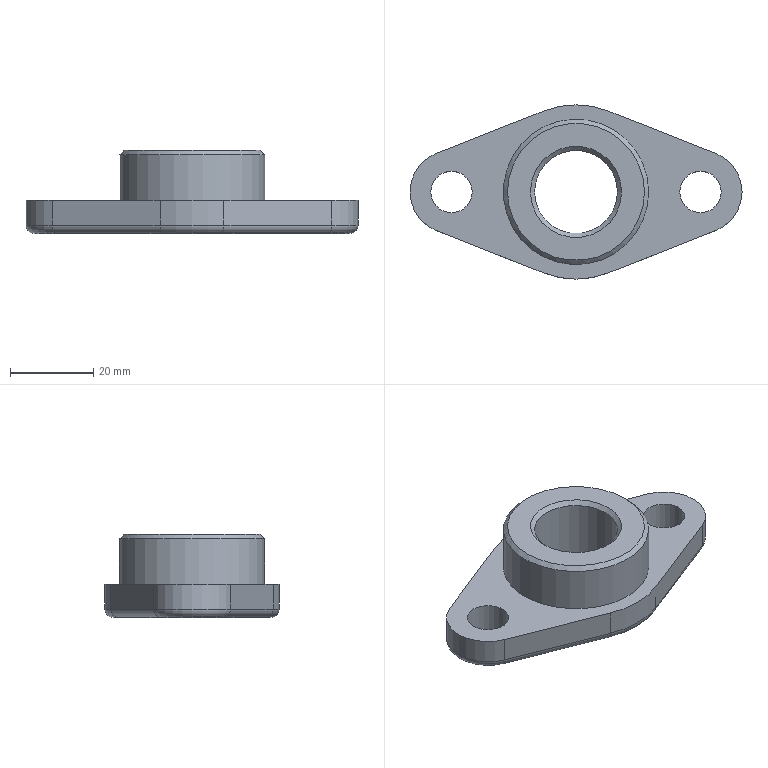Part | NX | features DATUM_CSYS 3, EXTRUDE 2, SKETCH 2, BLEND 1, CHAMFER 1, REPLACE_FACE 1 | 1 solid | 28 faces | box 80 x 42 x 20 mm | volume 22097 mm3 | cylinder 12 | plane 7 | cone 5 | torus 4 | commonest cylinder face diameters 4 x4 20 x3 10 x2 42 x2 35 x1
STEP:
#1=CARTESIAN_POINT('',(32.933,7.443,0.));
#2=VERTEX_POINT('',#1);
#3=CARTESIAN_POINT('',(32.933,-7.443,0.));
#4=VERTEX_POINT('',#3);
#5=CARTESIAN_POINT('',(30.,0.,0.));
#6=DIRECTION('',(0.,0.,1.));
#7=DIRECTION('',(1.,0.,0.));
#8=AXIS2_PLACEMENT_3D('',#5,#6,#7);
#9=CIRCLE('',#8,8.);
#10=EDGE_CURVE('',#2,#4,#9,.F.);
#11=ORIENTED_EDGE('',*,*,#10,.T.);
#12=CARTESIAN_POINT('',(6.967,-17.677,0.));
#13=VERTEX_POINT('',#12);
#14=CARTESIAN_POINT('',(-19.,-27.911,0.));
#15=DIRECTION('',(0.9304,0.3667,0.));
#16=VECTOR('',#15,1000.);
#17=LINE('',#14,#16);
#18=EDGE_CURVE('',#4,#13,#17,.F.);
#19=ORIENTED_EDGE('',*,*,#18,.T.);
#20=CARTESIAN_POINT('',(-6.967,-17.677,0.));
#21=VERTEX_POINT('',#20);
#22=CARTESIAN_POINT('',(0.,0.,0.));
#23=DIRECTION('',(0.,0.,1.));
#24=DIRECTION('',(1.,0.,0.));
#25=AXIS2_PLACEMENT_3D('',#22,#23,#24);
#26=CIRCLE('',#25,19.);
#27=EDGE_CURVE('',#13,#21,#26,.F.);
#28=ORIENTED_EDGE('',*,*,#27,.T.);
#29=CARTESIAN_POINT('',(-32.933,-7.443,0.));
#30=VERTEX_POINT('',#29);
#31=CARTESIAN_POINT('',(-32.933,-7.443,0.));
#32=DIRECTION('',(0.9304,-0.3667,0.));
#33=VECTOR('',#32,1000.);
#34=LINE('',#31,#33);
#35=EDGE_CURVE('',#21,#30,#34,.F.);
#36=ORIENTED_EDGE('',*,*,#35,.T.);
#37=CARTESIAN_POINT('',(-32.933,7.443,0.));
#38=VERTEX_POINT('',#37);
#39=CARTESIAN_POINT('',(-30.,0.,0.));
#40=DIRECTION('',(0.,0.,1.));
#41=DIRECTION('',(1.,0.,0.));
#42=AXIS2_PLACEMENT_3D('',#39,#40,#41);
#43=CIRCLE('',#42,8.);
#44=EDGE_CURVE('',#30,#38,#43,.F.);
#45=ORIENTED_EDGE('',*,*,#44,.T.);
#46=CARTESIAN_POINT('',(-6.967,17.677,0.));
#47=VERTEX_POINT('',#46);
#48=CARTESIAN_POINT('',(-32.933,7.443,0.));
#49=DIRECTION('',(-0.9304,-0.3667,0.));
#50=VECTOR('',#49,1000.);
#51=LINE('',#48,#50);
#52=EDGE_CURVE('',#38,#47,#51,.F.);
#53=ORIENTED_EDGE('',*,*,#52,.T.);
#54=CARTESIAN_POINT('',(6.967,17.677,0.));
#55=VERTEX_POINT('',#54);
#56=CARTESIAN_POINT('',(0.,0.,0.));
#57=DIRECTION('',(0.,0.,1.));
#58=DIRECTION('',(1.,0.,0.));
#59=AXIS2_PLACEMENT_3D('',#56,#57,#58);
#60=CIRCLE('',#59,19.);
#61=EDGE_CURVE('',#47,#55,#60,.F.);
#62=ORIENTED_EDGE('',*,*,#61,.T.);
#63=CARTESIAN_POINT('',(-19.,27.911,0.));
#64=DIRECTION('',(-0.9304,0.3667,0.));
#65=VECTOR('',#64,1000.);
#66=LINE('',#63,#65);
#67=EDGE_CURVE('',#55,#2,#66,.F.);
#68=ORIENTED_EDGE('',*,*,#67,.T.);
#69=EDGE_LOOP('',(#11,#19,#28,#36,#45,#53,#62,#68));
#70=FACE_BOUND('',#69,.T.);
#71=CARTESIAN_POINT('',(11.,0.,0.));
#72=VERTEX_POINT('',#71);
#73=CARTESIAN_POINT('',(0.,0.,0.));
#74=DIRECTION('',(0.,0.,1.));
#75=DIRECTION('',(1.,0.,0.));
#76=AXIS2_PLACEMENT_3D('',#73,#74,#75);
#77=CIRCLE('',#76,11.);
#78=EDGE_CURVE('',#72,#72,#77,.T.);
#79=ORIENTED_EDGE('',*,*,#78,.T.);
#80=EDGE_LOOP('',(#79));
#81=FACE_BOUND('',#80,.T.);
#82=CARTESIAN_POINT('',(36.,0.,0.));
#83=VERTEX_POINT('',#82);
#84=CARTESIAN_POINT('',(30.,0.,0.));
#85=DIRECTION('',(0.,0.,1.));
#86=DIRECTION('',(1.,0.,0.));
#87=AXIS2_PLACEMENT_3D('',#84,#85,#86);
#88=CIRCLE('',#87,6.);
#89=EDGE_CURVE('',#83,#83,#88,.T.);
#90=ORIENTED_EDGE('',*,*,#89,.T.);
#91=EDGE_LOOP('',(#90));
#92=FACE_BOUND('',#91,.T.);
#93=CARTESIAN_POINT('',(-24.,0.,0.));
#94=VERTEX_POINT('',#93);
#95=CARTESIAN_POINT('',(-30.,0.,0.));
#96=DIRECTION('',(0.,0.,1.));
#97=DIRECTION('',(1.,0.,0.));
#98=AXIS2_PLACEMENT_3D('',#95,#96,#97);
#99=CIRCLE('',#98,6.);
#100=EDGE_CURVE('',#94,#94,#99,.T.);
#101=ORIENTED_EDGE('',*,*,#100,.T.);
#102=EDGE_LOOP('',(#101));
#103=FACE_BOUND('',#102,.T.);
#104=CARTESIAN_POINT('',(-30.,0.,0.));
#105=DIRECTION('',(0.,0.,1.));
#106=DIRECTION('',(1.,0.,0.));
#107=AXIS2_PLACEMENT_3D('',#104,#105,#106);
#108=PLANE('',#107);
#109=ADVANCED_FACE('',(#70,#81,#92,#103),#108,.F.);
#110=CARTESIAN_POINT('',(-33.667,9.304,8.));
#111=VERTEX_POINT('',#110);
#112=CARTESIAN_POINT('',(-33.667,9.304,2.));
#113=VERTEX_POINT('',#112);
#114=CARTESIAN_POINT('',(-33.667,9.304,8.));
#115=DIRECTION('',(0.,0.,-1.));
#116=VECTOR('',#115,1000.);
#117=LINE('',#114,#116);
#118=EDGE_CURVE('',#111,#113,#117,.T.);
#119=ORIENTED_EDGE('',*,*,#118,.T.);
#120=CARTESIAN_POINT('',(-33.667,-9.304,2.));
#121=VERTEX_POINT('',#120);
#122=CARTESIAN_POINT('',(-30.,0.,2.));
#123=DIRECTION('',(0.,0.,1.));
#124=DIRECTION('',(1.,0.,0.));
#125=AXIS2_PLACEMENT_3D('',#122,#123,#124);
#126=CIRCLE('',#125,10.);
#127=EDGE_CURVE('',#113,#121,#126,.T.);
#128=ORIENTED_EDGE('',*,*,#127,.T.);
#129=CARTESIAN_POINT('',(-33.667,-9.304,8.));
#130=VERTEX_POINT('',#129);
#131=CARTESIAN_POINT('',(-33.667,-9.304,8.));
#132=DIRECTION('',(0.,0.,-1.));
#133=VECTOR('',#132,1000.);
#134=LINE('',#131,#133);
#135=EDGE_CURVE('',#130,#121,#134,.T.);
#136=ORIENTED_EDGE('',*,*,#135,.F.);
#137=CARTESIAN_POINT('',(-30.,0.,8.));
#138=DIRECTION('',(0.,0.,1.));
#139=DIRECTION('',(1.,0.,0.));
#140=AXIS2_PLACEMENT_3D('',#137,#138,#139);
#141=CIRCLE('',#140,10.);
#142=EDGE_CURVE('',#111,#130,#141,.T.);
#143=ORIENTED_EDGE('',*,*,#142,.F.);
#144=EDGE_LOOP('',(#119,#128,#136,#143));
#145=FACE_BOUND('',#144,.T.);
#146=CARTESIAN_POINT('',(-30.,0.,8.));
#147=DIRECTION('',(0.,0.,-1.));
#148=DIRECTION('',(-1.,0.,0.));
#149=AXIS2_PLACEMENT_3D('',#146,#147,#148);
#150=CYLINDRICAL_SURFACE('',#149,10.);
#151=ADVANCED_FACE('',(#145),#150,.T.);
#152=ORIENTED_EDGE('',*,*,#135,.T.);
#153=CARTESIAN_POINT('',(-7.7,-19.537,2.));
#154=VERTEX_POINT('',#153);
#155=CARTESIAN_POINT('',(-33.667,-9.304,2.));
#156=DIRECTION('',(0.9304,-0.3667,0.));
#157=VECTOR('',#156,1000.);
#158=LINE('',#155,#157);
#159=EDGE_CURVE('',#121,#154,#158,.T.);
#160=ORIENTED_EDGE('',*,*,#159,.T.);
#161=CARTESIAN_POINT('',(-7.7,-19.537,8.));
#162=VERTEX_POINT('',#161);
#163=CARTESIAN_POINT('',(-7.7,-19.537,8.));
#164=DIRECTION('',(0.,0.,-1.));
#165=VECTOR('',#164,1000.);
#166=LINE('',#163,#165);
#167=EDGE_CURVE('',#162,#154,#166,.T.);
#168=ORIENTED_EDGE('',*,*,#167,.F.);
#169=CARTESIAN_POINT('',(-33.667,-9.304,8.));
#170=DIRECTION('',(0.9304,-0.3667,0.));
#171=VECTOR('',#170,1000.);
#172=LINE('',#169,#171);
#173=EDGE_CURVE('',#130,#162,#172,.T.);
#174=ORIENTED_EDGE('',*,*,#173,.F.);
#175=EDGE_LOOP('',(#152,#160,#168,#174));
#176=FACE_BOUND('',#175,.T.);
#177=CARTESIAN_POINT('',(-33.667,-9.304,8.));
#178=DIRECTION('',(0.3667,0.9304,0.));
#179=DIRECTION('',(-0.9304,0.3667,0.));
#180=AXIS2_PLACEMENT_3D('',#177,#178,#179);
#181=PLANE('',#180);
#182=ADVANCED_FACE('',(#176),#181,.F.);
#183=ORIENTED_EDGE('',*,*,#167,.T.);
#184=CARTESIAN_POINT('',(7.7,-19.537,2.));
#185=VERTEX_POINT('',#184);
#186=CARTESIAN_POINT('',(0.,0.,2.));
#187=DIRECTION('',(0.,0.,1.));
#188=DIRECTION('',(1.,0.,0.));
#189=AXIS2_PLACEMENT_3D('',#186,#187,#188);
#190=CIRCLE('',#189,21.);
#191=EDGE_CURVE('',#154,#185,#190,.T.);
#192=ORIENTED_EDGE('',*,*,#191,.T.);
#193=CARTESIAN_POINT('',(7.7,-19.537,8.));
#194=VERTEX_POINT('',#193);
#195=CARTESIAN_POINT('',(7.7,-19.537,8.));
#196=DIRECTION('',(0.,0.,-1.));
#197=VECTOR('',#196,1000.);
#198=LINE('',#195,#197);
#199=EDGE_CURVE('',#194,#185,#198,.T.);
#200=ORIENTED_EDGE('',*,*,#199,.F.);
#201=CARTESIAN_POINT('',(0.,0.,8.));
#202=DIRECTION('',(0.,0.,1.));
#203=DIRECTION('',(1.,0.,0.));
#204=AXIS2_PLACEMENT_3D('',#201,#202,#203);
#205=CIRCLE('',#204,21.);
#206=EDGE_CURVE('',#162,#194,#205,.T.);
#207=ORIENTED_EDGE('',*,*,#206,.F.);
#208=EDGE_LOOP('',(#183,#192,#200,#207));
#209=FACE_BOUND('',#208,.T.);
#210=CARTESIAN_POINT('',(0.,0.,8.));
#211=DIRECTION('',(0.,0.,-1.));
#212=DIRECTION('',(-1.,0.,0.));
#213=AXIS2_PLACEMENT_3D('',#210,#211,#212);
#214=CYLINDRICAL_SURFACE('',#213,21.);
#215=ADVANCED_FACE('',(#209),#214,.T.);
#216=ORIENTED_EDGE('',*,*,#199,.T.);
#217=CARTESIAN_POINT('',(33.667,-9.304,2.));
#218=VERTEX_POINT('',#217);
#219=CARTESIAN_POINT('',(7.7,-19.537,2.));
#220=DIRECTION('',(0.9304,0.3667,0.));
#221=VECTOR('',#220,1000.);
#222=LINE('',#219,#221);
#223=EDGE_CURVE('',#185,#218,#222,.T.);
#224=ORIENTED_EDGE('',*,*,#223,.T.);
#225=CARTESIAN_POINT('',(33.667,-9.304,8.));
#226=VERTEX_POINT('',#225);
#227=CARTESIAN_POINT('',(33.667,-9.304,8.));
#228=DIRECTION('',(0.,0.,-1.));
#229=VECTOR('',#228,1000.);
#230=LINE('',#227,#229);
#231=EDGE_CURVE('',#226,#218,#230,.T.);
#232=ORIENTED_EDGE('',*,*,#231,.F.);
#233=CARTESIAN_POINT('',(7.7,-19.537,8.));
#234=DIRECTION('',(0.9304,0.3667,0.));
#235=VECTOR('',#234,1000.);
#236=LINE('',#233,#235);
#237=EDGE_CURVE('',#194,#226,#236,.T.);
#238=ORIENTED_EDGE('',*,*,#237,.F.);
#239=EDGE_LOOP('',(#216,#224,#232,#238));
#240=FACE_BOUND('',#239,.T.);
#241=CARTESIAN_POINT('',(7.7,-19.537,8.));
#242=DIRECTION('',(-0.3667,0.9304,0.));
#243=DIRECTION('',(-0.9304,-0.3667,0.));
#244=AXIS2_PLACEMENT_3D('',#241,#242,#243);
#245=PLANE('',#244);
#246=ADVANCED_FACE('',(#240),#245,.F.);
#247=ORIENTED_EDGE('',*,*,#231,.T.);
#248=CARTESIAN_POINT('',(33.667,9.304,2.));
#249=VERTEX_POINT('',#248);
#250=CARTESIAN_POINT('',(30.,0.,2.));
#251=DIRECTION('',(0.,0.,1.));
#252=DIRECTION('',(1.,0.,0.));
#253=AXIS2_PLACEMENT_3D('',#250,#251,#252);
#254=CIRCLE('',#253,10.);
#255=EDGE_CURVE('',#218,#249,#254,.T.);
#256=ORIENTED_EDGE('',*,*,#255,.T.);
#257=CARTESIAN_POINT('',(33.667,9.304,8.));
#258=VERTEX_POINT('',#257);
#259=CARTESIAN_POINT('',(33.667,9.304,8.));
#260=DIRECTION('',(0.,0.,-1.));
#261=VECTOR('',#260,1000.);
#262=LINE('',#259,#261);
#263=EDGE_CURVE('',#258,#249,#262,.T.);
#264=ORIENTED_EDGE('',*,*,#263,.F.);
#265=CARTESIAN_POINT('',(30.,0.,8.));
#266=DIRECTION('',(0.,0.,1.));
#267=DIRECTION('',(1.,0.,0.));
#268=AXIS2_PLACEMENT_3D('',#265,#266,#267);
#269=CIRCLE('',#268,10.);
#270=EDGE_CURVE('',#226,#258,#269,.T.);
#271=ORIENTED_EDGE('',*,*,#270,.F.);
#272=EDGE_LOOP('',(#247,#256,#264,#271));
#273=FACE_BOUND('',#272,.T.);
#274=CARTESIAN_POINT('',(30.,0.,8.));
#275=DIRECTION('',(0.,0.,-1.));
#276=DIRECTION('',(-1.,0.,0.));
#277=AXIS2_PLACEMENT_3D('',#274,#275,#276);
#278=CYLINDRICAL_SURFACE('',#277,10.);
#279=ADVANCED_FACE('',(#273),#278,.T.);
#280=ORIENTED_EDGE('',*,*,#263,.T.);
#281=CARTESIAN_POINT('',(7.7,19.537,2.));
#282=VERTEX_POINT('',#281);
#283=CARTESIAN_POINT('',(33.667,9.304,2.));
#284=DIRECTION('',(-0.9304,0.3667,0.));
#285=VECTOR('',#284,1000.);
#286=LINE('',#283,#285);
#287=EDGE_CURVE('',#249,#282,#286,.T.);
#288=ORIENTED_EDGE('',*,*,#287,.T.);
#289=CARTESIAN_POINT('',(7.7,19.537,8.));
#290=VERTEX_POINT('',#289);
#291=CARTESIAN_POINT('',(7.7,19.537,8.));
#292=DIRECTION('',(0.,0.,-1.));
#293=VECTOR('',#292,1000.);
#294=LINE('',#291,#293);
#295=EDGE_CURVE('',#290,#282,#294,.T.);
#296=ORIENTED_EDGE('',*,*,#295,.F.);
#297=CARTESIAN_POINT('',(33.667,9.304,8.));
#298=DIRECTION('',(-0.9304,0.3667,0.));
#299=VECTOR('',#298,1000.);
#300=LINE('',#297,#299);
#301=EDGE_CURVE('',#258,#290,#300,.T.);
#302=ORIENTED_EDGE('',*,*,#301,.F.);
#303=EDGE_LOOP('',(#280,#288,#296,#302));
#304=FACE_BOUND('',#303,.T.);
#305=CARTESIAN_POINT('',(33.667,9.304,8.));
#306=DIRECTION('',(-0.3667,-0.9304,0.));
#307=DIRECTION('',(0.9304,-0.3667,0.));
#308=AXIS2_PLACEMENT_3D('',#305,#306,#307);
#309=PLANE('',#308);
#310=ADVANCED_FACE('',(#304),#309,.F.);
#311=ORIENTED_EDGE('',*,*,#295,.T.);
#312=CARTESIAN_POINT('',(-7.7,19.537,2.));
#313=VERTEX_POINT('',#312);
#314=CARTESIAN_POINT('',(0.,0.,2.));
#315=DIRECTION('',(0.,0.,1.));
#316=DIRECTION('',(1.,0.,0.));
#317=AXIS2_PLACEMENT_3D('',#314,#315,#316);
#318=CIRCLE('',#317,21.);
#319=EDGE_CURVE('',#282,#313,#318,.T.);
#320=ORIENTED_EDGE('',*,*,#319,.T.);
#321=CARTESIAN_POINT('',(-7.7,19.537,8.));
#322=VERTEX_POINT('',#321);
#323=CARTESIAN_POINT('',(-7.7,19.537,8.));
#324=DIRECTION('',(0.,0.,-1.));
#325=VECTOR('',#324,1000.);
#326=LINE('',#323,#325);
#327=EDGE_CURVE('',#322,#313,#326,.T.);
#328=ORIENTED_EDGE('',*,*,#327,.F.);
#329=CARTESIAN_POINT('',(0.,0.,8.));
#330=DIRECTION('',(0.,0.,1.));
#331=DIRECTION('',(1.,0.,0.));
#332=AXIS2_PLACEMENT_3D('',#329,#330,#331);
#333=CIRCLE('',#332,21.);
#334=EDGE_CURVE('',#290,#322,#333,.T.);
#335=ORIENTED_EDGE('',*,*,#334,.F.);
#336=EDGE_LOOP('',(#311,#320,#328,#335));
#337=FACE_BOUND('',#336,.T.);
#338=CARTESIAN_POINT('',(0.,0.,8.));
#339=DIRECTION('',(0.,0.,-1.));
#340=DIRECTION('',(-1.,0.,0.));
#341=AXIS2_PLACEMENT_3D('',#338,#339,#340);
#342=CYLINDRICAL_SURFACE('',#341,21.);
#343=ADVANCED_FACE('',(#337),#342,.T.);
#344=CARTESIAN_POINT('',(-25.,0.,1.));
#345=VERTEX_POINT('',#344);
#346=CARTESIAN_POINT('',(-30.,0.,1.));
#347=DIRECTION('',(0.,0.,1.));
#348=DIRECTION('',(1.,0.,0.));
#349=AXIS2_PLACEMENT_3D('',#346,#347,#348);
#350=CIRCLE('',#349,5.);
#351=EDGE_CURVE('',#345,#345,#350,.F.);
#352=ORIENTED_EDGE('',*,*,#351,.T.);
#353=EDGE_LOOP('',(#352));
#354=FACE_BOUND('',#353,.T.);
#355=CARTESIAN_POINT('',(-25.,0.,8.));
#356=VERTEX_POINT('',#355);
#357=CARTESIAN_POINT('',(-30.,0.,8.));
#358=DIRECTION('',(0.,0.,1.));
#359=DIRECTION('',(1.,0.,0.));
#360=AXIS2_PLACEMENT_3D('',#357,#358,#359);
#361=CIRCLE('',#360,5.);
#362=EDGE_CURVE('',#356,#356,#361,.T.);
#363=ORIENTED_EDGE('',*,*,#362,.T.);
#364=EDGE_LOOP('',(#363));
#365=FACE_BOUND('',#364,.T.);
#366=CARTESIAN_POINT('',(-30.,0.,8.));
#367=DIRECTION('',(0.,0.,-1.));
#368=DIRECTION('',(-1.,0.,0.));
#369=AXIS2_PLACEMENT_3D('',#366,#367,#368);
#370=CYLINDRICAL_SURFACE('',#369,5.);
#371=ADVANCED_FACE('',(#354,#365),#370,.F.);
#372=ORIENTED_EDGE('',*,*,#327,.T.);
#373=CARTESIAN_POINT('',(-7.7,19.537,2.));
#374=DIRECTION('',(-0.9304,-0.3667,0.));
#375=VECTOR('',#374,1000.);
#376=LINE('',#373,#375);
#377=EDGE_CURVE('',#313,#113,#376,.T.);
#378=ORIENTED_EDGE('',*,*,#377,.T.);
#379=ORIENTED_EDGE('',*,*,#118,.F.);
#380=CARTESIAN_POINT('',(-7.7,19.537,8.));
#381=DIRECTION('',(-0.9304,-0.3667,0.));
#382=VECTOR('',#381,1000.);
#383=LINE('',#380,#382);
#384=EDGE_CURVE('',#322,#111,#383,.T.);
#385=ORIENTED_EDGE('',*,*,#384,.F.);
#386=EDGE_LOOP('',(#372,#378,#379,#385));
#387=FACE_BOUND('',#386,.T.);
#388=CARTESIAN_POINT('',(-7.7,19.537,8.));
#389=DIRECTION('',(0.3667,-0.9304,0.));
#390=DIRECTION('',(0.9304,0.3667,0.));
#391=AXIS2_PLACEMENT_3D('',#388,#389,#390);
#392=PLANE('',#391);
#393=ADVANCED_FACE('',(#387),#392,.F.);
#394=CARTESIAN_POINT('',(35.,0.,1.));
#395=VERTEX_POINT('',#394);
#396=CARTESIAN_POINT('',(30.,0.,1.));
#397=DIRECTION('',(0.,0.,1.));
#398=DIRECTION('',(1.,0.,0.));
#399=AXIS2_PLACEMENT_3D('',#396,#397,#398);
#400=CIRCLE('',#399,5.);
#401=EDGE_CURVE('',#395,#395,#400,.F.);
#402=ORIENTED_EDGE('',*,*,#401,.T.);
#403=EDGE_LOOP('',(#402));
#404=FACE_BOUND('',#403,.T.);
#405=CARTESIAN_POINT('',(35.,0.,8.));
#406=VERTEX_POINT('',#405);
#407=CARTESIAN_POINT('',(30.,0.,8.));
#408=DIRECTION('',(0.,0.,1.));
#409=DIRECTION('',(1.,0.,0.));
#410=AXIS2_PLACEMENT_3D('',#407,#408,#409);
#411=CIRCLE('',#410,5.);
#412=EDGE_CURVE('',#406,#406,#411,.T.);
#413=ORIENTED_EDGE('',*,*,#412,.T.);
#414=EDGE_LOOP('',(#413));
#415=FACE_BOUND('',#414,.T.);
#416=CARTESIAN_POINT('',(30.,0.,8.));
#417=DIRECTION('',(0.,0.,-1.));
#418=DIRECTION('',(-1.,0.,0.));
#419=AXIS2_PLACEMENT_3D('',#416,#417,#418);
#420=CYLINDRICAL_SURFACE('',#419,5.);
#421=ADVANCED_FACE('',(#404,#415),#420,.F.);
#422=CARTESIAN_POINT('',(17.5,0.,8.));
#423=VERTEX_POINT('',#422);
#424=CARTESIAN_POINT('',(0.,0.,8.));
#425=DIRECTION('',(0.,0.,1.));
#426=DIRECTION('',(1.,0.,0.));
#427=AXIS2_PLACEMENT_3D('',#424,#425,#426);
#428=CIRCLE('',#427,17.5);
#429=EDGE_CURVE('',#423,#423,#428,.F.);
#430=ORIENTED_EDGE('',*,*,#429,.T.);
#431=EDGE_LOOP('',(#430));
#432=FACE_BOUND('',#431,.T.);
#433=ORIENTED_EDGE('',*,*,#142,.T.);
#434=ORIENTED_EDGE('',*,*,#173,.T.);
#435=ORIENTED_EDGE('',*,*,#206,.T.);
#436=ORIENTED_EDGE('',*,*,#237,.T.);
#437=ORIENTED_EDGE('',*,*,#270,.T.);
#438=ORIENTED_EDGE('',*,*,#301,.T.);
#439=ORIENTED_EDGE('',*,*,#334,.T.);
#440=ORIENTED_EDGE('',*,*,#384,.T.);
#441=EDGE_LOOP('',(#433,#434,#435,#436,#437,#438,#439,#440));
#442=FACE_BOUND('',#441,.T.);
#443=ORIENTED_EDGE('',*,*,#362,.F.);
#444=EDGE_LOOP('',(#443));
#445=FACE_BOUND('',#444,.T.);
#446=ORIENTED_EDGE('',*,*,#412,.F.);
#447=EDGE_LOOP('',(#446));
#448=FACE_BOUND('',#447,.T.);
#449=CARTESIAN_POINT('',(-30.,0.,8.));
#450=DIRECTION('',(0.,0.,1.));
#451=DIRECTION('',(1.,0.,0.));
#452=AXIS2_PLACEMENT_3D('',#449,#450,#451);
#453=PLANE('',#452);
#454=ADVANCED_FACE('',(#432,#442,#445,#448),#453,.T.);
#455=CARTESIAN_POINT('',(17.5,0.,19.));
#456=VERTEX_POINT('',#455);
#457=CARTESIAN_POINT('',(0.,0.,19.));
#458=DIRECTION('',(0.,0.,1.));
#459=DIRECTION('',(1.,0.,0.));
#460=AXIS2_PLACEMENT_3D('',#457,#458,#459);
#461=CIRCLE('',#460,17.5);
#462=EDGE_CURVE('',#456,#456,#461,.F.);
#463=ORIENTED_EDGE('',*,*,#462,.T.);
#464=EDGE_LOOP('',(#463));
#465=FACE_BOUND('',#464,.T.);
#466=ORIENTED_EDGE('',*,*,#429,.F.);
#467=EDGE_LOOP('',(#466));
#468=FACE_BOUND('',#467,.T.);
#469=CARTESIAN_POINT('',(0.,0.,20.));
#470=DIRECTION('',(0.,0.,-1.));
#471=DIRECTION('',(-1.,0.,0.));
#472=AXIS2_PLACEMENT_3D('',#469,#470,#471);
#473=CYLINDRICAL_SURFACE('',#472,17.5);
#474=ADVANCED_FACE('',(#465,#468),#473,.T.);
#475=CARTESIAN_POINT('',(10.,0.,19.));
#476=VERTEX_POINT('',#475);
#477=CARTESIAN_POINT('',(0.,0.,19.));
#478=DIRECTION('',(0.,0.,1.));
#479=DIRECTION('',(1.,0.,0.));
#480=AXIS2_PLACEMENT_3D('',#477,#478,#479);
#481=CIRCLE('',#480,10.);
#482=EDGE_CURVE('',#476,#476,#481,.T.);
#483=ORIENTED_EDGE('',*,*,#482,.T.);
#484=EDGE_LOOP('',(#483));
#485=FACE_BOUND('',#484,.T.);
#486=CARTESIAN_POINT('',(10.,0.,1.));
#487=VERTEX_POINT('',#486);
#488=CARTESIAN_POINT('',(0.,0.,1.));
#489=DIRECTION('',(0.,0.,1.));
#490=DIRECTION('',(1.,0.,0.));
#491=AXIS2_PLACEMENT_3D('',#488,#489,#490);
#492=CIRCLE('',#491,10.);
#493=EDGE_CURVE('',#487,#487,#492,.F.);
#494=ORIENTED_EDGE('',*,*,#493,.T.);
#495=EDGE_LOOP('',(#494));
#496=FACE_BOUND('',#495,.T.);
#497=CARTESIAN_POINT('',(0.,0.,20.));
#498=DIRECTION('',(0.,0.,-1.));
#499=DIRECTION('',(-1.,0.,0.));
#500=AXIS2_PLACEMENT_3D('',#497,#498,#499);
#501=CYLINDRICAL_SURFACE('',#500,10.);
#502=ADVANCED_FACE('',(#485,#496),#501,.F.);
#503=CARTESIAN_POINT('',(11.,0.,20.));
#504=VERTEX_POINT('',#503);
#505=CARTESIAN_POINT('',(0.,0.,20.));
#506=DIRECTION('',(0.,0.,1.));
#507=DIRECTION('',(1.,0.,0.));
#508=AXIS2_PLACEMENT_3D('',#505,#506,#507);
#509=CIRCLE('',#508,11.);
#510=EDGE_CURVE('',#504,#504,#509,.F.);
#511=ORIENTED_EDGE('',*,*,#510,.T.);
#512=EDGE_LOOP('',(#511));
#513=FACE_BOUND('',#512,.T.);
#514=CARTESIAN_POINT('',(16.5,0.,20.));
#515=VERTEX_POINT('',#514);
#516=CARTESIAN_POINT('',(0.,0.,20.));
#517=DIRECTION('',(0.,0.,1.));
#518=DIRECTION('',(1.,0.,0.));
#519=AXIS2_PLACEMENT_3D('',#516,#517,#518);
#520=CIRCLE('',#519,16.5);
#521=EDGE_CURVE('',#515,#515,#520,.T.);
#522=ORIENTED_EDGE('',*,*,#521,.T.);
#523=EDGE_LOOP('',(#522));
#524=FACE_BOUND('',#523,.T.);
#525=CARTESIAN_POINT('',(0.,0.,20.));
#526=DIRECTION('',(0.,0.,1.));
#527=DIRECTION('',(1.,0.,0.));
#528=AXIS2_PLACEMENT_3D('',#525,#526,#527);
#529=PLANE('',#528);
#530=ADVANCED_FACE('',(#513,#524),#529,.T.);
#531=ORIENTED_EDGE('',*,*,#510,.F.);
#532=EDGE_LOOP('',(#531));
#533=FACE_BOUND('',#532,.T.);
#534=ORIENTED_EDGE('',*,*,#482,.F.);
#535=EDGE_LOOP('',(#534));
#536=FACE_BOUND('',#535,.T.);
#537=CARTESIAN_POINT('',(0.,0.,19.));
#538=DIRECTION('',(0.,0.,1.));
#539=DIRECTION('',(1.,0.,0.));
#540=AXIS2_PLACEMENT_3D('',#537,#538,#539);
#541=CONICAL_SURFACE('',#540,10.,0.7854);
#542=ADVANCED_FACE('',(#533,#536),#541,.F.);
#543=ORIENTED_EDGE('',*,*,#462,.F.);
#544=EDGE_LOOP('',(#543));
#545=FACE_BOUND('',#544,.T.);
#546=ORIENTED_EDGE('',*,*,#521,.F.);
#547=EDGE_LOOP('',(#546));
#548=FACE_BOUND('',#547,.T.);
#549=CARTESIAN_POINT('',(0.,0.,20.));
#550=DIRECTION('',(0.,0.,-1.));
#551=DIRECTION('',(-1.,0.,0.));
#552=AXIS2_PLACEMENT_3D('',#549,#550,#551);
#553=CONICAL_SURFACE('',#552,16.5,0.7854);
#554=ADVANCED_FACE('',(#545,#548),#553,.T.);
#555=ORIENTED_EDGE('',*,*,#78,.F.);
#556=EDGE_LOOP('',(#555));
#557=FACE_BOUND('',#556,.T.);
#558=ORIENTED_EDGE('',*,*,#493,.F.);
#559=EDGE_LOOP('',(#558));
#560=FACE_BOUND('',#559,.T.);
#561=CARTESIAN_POINT('',(0.,0.,1.));
#562=DIRECTION('',(0.,0.,-1.));
#563=DIRECTION('',(-1.,0.,0.));
#564=AXIS2_PLACEMENT_3D('',#561,#562,#563);
#565=CONICAL_SURFACE('',#564,10.,0.7854);
#566=ADVANCED_FACE('',(#557,#560),#565,.F.);
#567=ORIENTED_EDGE('',*,*,#401,.F.);
#568=EDGE_LOOP('',(#567));
#569=FACE_BOUND('',#568,.T.);
#570=ORIENTED_EDGE('',*,*,#89,.F.);
#571=EDGE_LOOP('',(#570));
#572=FACE_BOUND('',#571,.T.);
#573=CARTESIAN_POINT('',(30.,0.,0.));
#574=DIRECTION('',(0.,0.,-1.));
#575=DIRECTION('',(-1.,0.,0.));
#576=AXIS2_PLACEMENT_3D('',#573,#574,#575);
#577=CONICAL_SURFACE('',#576,6.,0.7854);
#578=ADVANCED_FACE('',(#569,#572),#577,.F.);
#579=ORIENTED_EDGE('',*,*,#351,.F.);
#580=EDGE_LOOP('',(#579));
#581=FACE_BOUND('',#580,.T.);
#582=ORIENTED_EDGE('',*,*,#100,.F.);
#583=EDGE_LOOP('',(#582));
#584=FACE_BOUND('',#583,.T.);
#585=CARTESIAN_POINT('',(-30.,0.,0.));
#586=DIRECTION('',(0.,0.,-1.));
#587=DIRECTION('',(-1.,0.,0.));
#588=AXIS2_PLACEMENT_3D('',#585,#586,#587);
#589=CONICAL_SURFACE('',#588,6.,0.7854);
#590=ADVANCED_FACE('',(#581,#584),#589,.F.);
#591=CARTESIAN_POINT('',(-32.933,7.443,2.));
#592=DIRECTION('',(0.9304,0.3667,0.));
#593=DIRECTION('',(-0.3667,0.9304,0.));
#594=AXIS2_PLACEMENT_3D('',#591,#592,#593);
#595=CIRCLE('',#594,2.);
#596=EDGE_CURVE('',#38,#113,#595,.T.);
#597=ORIENTED_EDGE('',*,*,#596,.F.);
#598=ORIENTED_EDGE('',*,*,#44,.F.);
#599=CARTESIAN_POINT('',(-32.933,-7.443,2.));
#600=DIRECTION('',(0.9304,-0.3667,0.));
#601=DIRECTION('',(0.3667,0.9304,0.));
#602=AXIS2_PLACEMENT_3D('',#599,#600,#601);
#603=CIRCLE('',#602,2.);
#604=EDGE_CURVE('',#121,#30,#603,.T.);
#605=ORIENTED_EDGE('',*,*,#604,.F.);
#606=ORIENTED_EDGE('',*,*,#127,.F.);
#607=EDGE_LOOP('',(#597,#598,#605,#606));
#608=FACE_BOUND('',#607,.T.);
#609=CARTESIAN_POINT('',(-30.,0.,2.));
#610=DIRECTION('',(0.,0.,1.));
#611=DIRECTION('',(1.,0.,0.));
#612=AXIS2_PLACEMENT_3D('',#609,#610,#611);
#613=TOROIDAL_SURFACE('',#612,8.,2.);
#614=ADVANCED_FACE('',(#608),#613,.T.);
#615=ORIENTED_EDGE('',*,*,#604,.T.);
#616=ORIENTED_EDGE('',*,*,#35,.F.);
#617=CARTESIAN_POINT('',(-6.967,-17.677,2.));
#618=DIRECTION('',(0.9304,-0.3667,0.));
#619=DIRECTION('',(0.3667,0.9304,0.));
#620=AXIS2_PLACEMENT_3D('',#617,#618,#619);
#621=CIRCLE('',#620,2.);
#622=EDGE_CURVE('',#154,#21,#621,.T.);
#623=ORIENTED_EDGE('',*,*,#622,.F.);
#624=ORIENTED_EDGE('',*,*,#159,.F.);
#625=EDGE_LOOP('',(#615,#616,#623,#624));
#626=FACE_BOUND('',#625,.T.);
#627=CARTESIAN_POINT('',(-32.933,-7.443,2.));
#628=DIRECTION('',(0.9304,-0.3667,0.));
#629=DIRECTION('',(0.3667,0.9304,0.));
#630=AXIS2_PLACEMENT_3D('',#627,#628,#629);
#631=CYLINDRICAL_SURFACE('',#630,2.);
#632=ADVANCED_FACE('',(#626),#631,.T.);
#633=ORIENTED_EDGE('',*,*,#596,.T.);
#634=ORIENTED_EDGE('',*,*,#377,.F.);
#635=CARTESIAN_POINT('',(-6.967,17.677,2.));
#636=DIRECTION('',(0.9304,0.3667,0.));
#637=DIRECTION('',(-0.3667,0.9304,0.));
#638=AXIS2_PLACEMENT_3D('',#635,#636,#637);
#639=CIRCLE('',#638,2.);
#640=EDGE_CURVE('',#47,#313,#639,.T.);
#641=ORIENTED_EDGE('',*,*,#640,.F.);
#642=ORIENTED_EDGE('',*,*,#52,.F.);
#643=EDGE_LOOP('',(#633,#634,#641,#642));
#644=FACE_BOUND('',#643,.T.);
#645=CARTESIAN_POINT('',(-6.967,17.677,2.));
#646=DIRECTION('',(-0.9304,-0.3667,0.));
#647=DIRECTION('',(0.3667,-0.9304,0.));
#648=AXIS2_PLACEMENT_3D('',#645,#646,#647);
#649=CYLINDRICAL_SURFACE('',#648,2.);
#650=ADVANCED_FACE('',(#644),#649,.T.);
#651=ORIENTED_EDGE('',*,*,#622,.T.);
#652=ORIENTED_EDGE('',*,*,#27,.F.);
#653=CARTESIAN_POINT('',(6.967,-17.677,2.));
#654=DIRECTION('',(0.9304,0.3667,0.));
#655=DIRECTION('',(-0.3667,0.9304,0.));
#656=AXIS2_PLACEMENT_3D('',#653,#654,#655);
#657=CIRCLE('',#656,2.);
#658=EDGE_CURVE('',#185,#13,#657,.T.);
#659=ORIENTED_EDGE('',*,*,#658,.F.);
#660=ORIENTED_EDGE('',*,*,#191,.F.);
#661=EDGE_LOOP('',(#651,#652,#659,#660));
#662=FACE_BOUND('',#661,.T.);
#663=CARTESIAN_POINT('',(0.,0.,2.));
#664=DIRECTION('',(0.,0.,1.));
#665=DIRECTION('',(1.,0.,0.));
#666=AXIS2_PLACEMENT_3D('',#663,#664,#665);
#667=TOROIDAL_SURFACE('',#666,19.,2.);
#668=ADVANCED_FACE('',(#662),#667,.T.);
#669=ORIENTED_EDGE('',*,*,#640,.T.);
#670=ORIENTED_EDGE('',*,*,#319,.F.);
#671=CARTESIAN_POINT('',(6.967,17.677,2.));
#672=DIRECTION('',(0.9304,-0.3667,0.));
#673=DIRECTION('',(0.3667,0.9304,0.));
#674=AXIS2_PLACEMENT_3D('',#671,#672,#673);
#675=CIRCLE('',#674,2.);
#676=EDGE_CURVE('',#55,#282,#675,.T.);
#677=ORIENTED_EDGE('',*,*,#676,.F.);
#678=ORIENTED_EDGE('',*,*,#61,.F.);
#679=EDGE_LOOP('',(#669,#670,#677,#678));
#680=FACE_BOUND('',#679,.T.);
#681=CARTESIAN_POINT('',(0.,0.,2.));
#682=DIRECTION('',(0.,0.,1.));
#683=DIRECTION('',(1.,0.,0.));
#684=AXIS2_PLACEMENT_3D('',#681,#682,#683);
#685=TOROIDAL_SURFACE('',#684,19.,2.);
#686=ADVANCED_FACE('',(#680),#685,.T.);
#687=ORIENTED_EDGE('',*,*,#658,.T.);
#688=ORIENTED_EDGE('',*,*,#18,.F.);
#689=CARTESIAN_POINT('',(32.933,-7.443,2.));
#690=DIRECTION('',(0.9304,0.3667,0.));
#691=DIRECTION('',(-0.3667,0.9304,0.));
#692=AXIS2_PLACEMENT_3D('',#689,#690,#691);
#693=CIRCLE('',#692,2.);
#694=EDGE_CURVE('',#218,#4,#693,.T.);
#695=ORIENTED_EDGE('',*,*,#694,.F.);
#696=ORIENTED_EDGE('',*,*,#223,.F.);
#697=EDGE_LOOP('',(#687,#688,#695,#696));
#698=FACE_BOUND('',#697,.T.);
#699=CARTESIAN_POINT('',(6.967,-17.677,2.));
#700=DIRECTION('',(0.9304,0.3667,0.));
#701=DIRECTION('',(-0.3667,0.9304,0.));
#702=AXIS2_PLACEMENT_3D('',#699,#700,#701);
#703=CYLINDRICAL_SURFACE('',#702,2.);
#704=ADVANCED_FACE('',(#698),#703,.T.);
#705=ORIENTED_EDGE('',*,*,#676,.T.);
#706=ORIENTED_EDGE('',*,*,#287,.F.);
#707=CARTESIAN_POINT('',(32.933,7.443,2.));
#708=DIRECTION('',(0.9304,-0.3667,0.));
#709=DIRECTION('',(0.3667,0.9304,0.));
#710=AXIS2_PLACEMENT_3D('',#707,#708,#709);
#711=CIRCLE('',#710,2.);
#712=EDGE_CURVE('',#2,#249,#711,.T.);
#713=ORIENTED_EDGE('',*,*,#712,.F.);
#714=ORIENTED_EDGE('',*,*,#67,.F.);
#715=EDGE_LOOP('',(#705,#706,#713,#714));
#716=FACE_BOUND('',#715,.T.);
#717=CARTESIAN_POINT('',(32.933,7.443,2.));
#718=DIRECTION('',(-0.9304,0.3667,0.));
#719=DIRECTION('',(-0.3667,-0.9304,0.));
#720=AXIS2_PLACEMENT_3D('',#717,#718,#719);
#721=CYLINDRICAL_SURFACE('',#720,2.);
#722=ADVANCED_FACE('',(#716),#721,.T.);
#723=ORIENTED_EDGE('',*,*,#694,.T.);
#724=ORIENTED_EDGE('',*,*,#10,.F.);
#725=ORIENTED_EDGE('',*,*,#712,.T.);
#726=ORIENTED_EDGE('',*,*,#255,.F.);
#727=EDGE_LOOP('',(#723,#724,#725,#726));
#728=FACE_BOUND('',#727,.T.);
#729=CARTESIAN_POINT('',(30.,0.,2.));
#730=DIRECTION('',(0.,0.,1.));
#731=DIRECTION('',(1.,0.,0.));
#732=AXIS2_PLACEMENT_3D('',#729,#730,#731);
#733=TOROIDAL_SURFACE('',#732,8.,2.);
#734=ADVANCED_FACE('',(#728),#733,.T.);
#735=CLOSED_SHELL('',(#109,#151,#182,#215,#246,#279,#310,#343,#371,#393,#421,#454,#474,#502,#530,#542,#554,#566,#578,#590,#614,#632,#650,#668,#686,#704,#722,#734));
#736=MANIFOLD_SOLID_BREP('',#735);
#737=(LENGTH_UNIT()NAMED_UNIT(*)SI_UNIT(.MILLI.,.METRE.));
#738=UNCERTAINTY_MEASURE_WITH_UNIT(LENGTH_MEASURE(0.00001),#737,'','');
#739=(NAMED_UNIT(*)PLANE_ANGLE_UNIT()SI_UNIT($,.RADIAN.));
#740=(NAMED_UNIT(*)SI_UNIT($,.STERADIAN.)SOLID_ANGLE_UNIT());
#741=(GEOMETRIC_REPRESENTATION_CONTEXT(3)GLOBAL_UNCERTAINTY_ASSIGNED_CONTEXT((#738))GLOBAL_UNIT_ASSIGNED_CONTEXT((#737,#739,#740))REPRESENTATION_CONTEXT('',''));
#742=ADVANCED_BREP_SHAPE_REPRESENTATION('',(#736),#741);